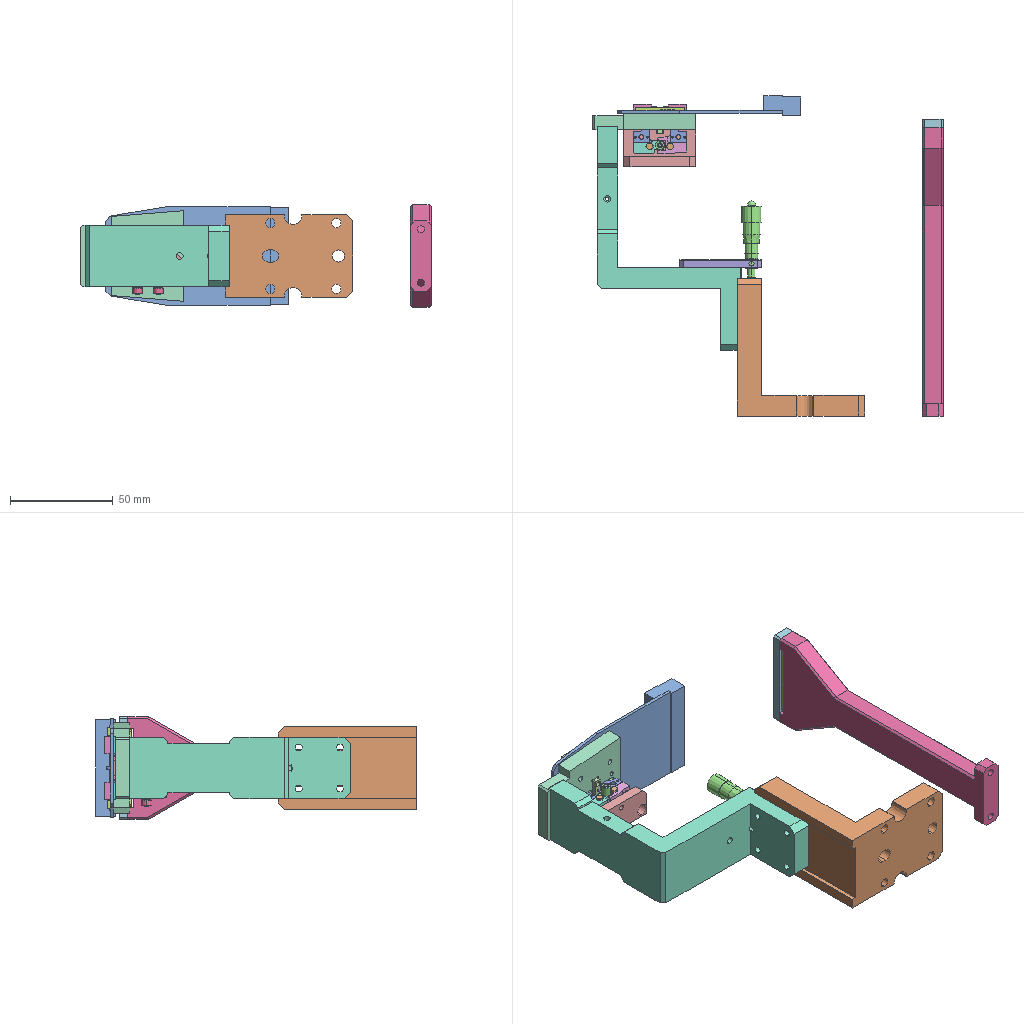Assembly | SolidWorks | 33 different items | 55 placed | box 170 x 156 x 50 mm
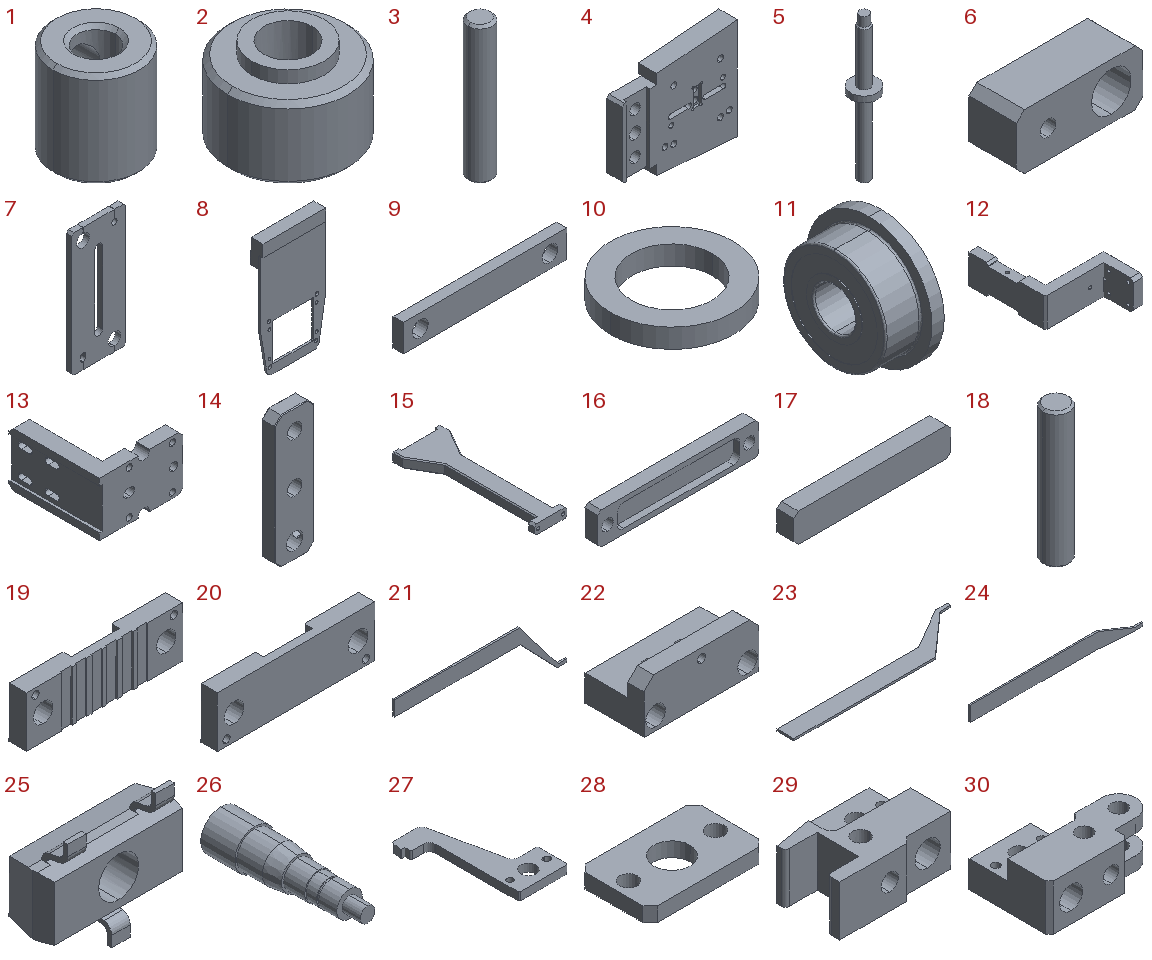Parts list (item | quantity | size | volume | features):
1 | x1 | 4.5 x 4.5 x 5 mm | 60.379 mm3 | features Chamfer 1, Extrusion 1, HoleWzd 1
2 | x2 | 5 x 5 x 3.5 mm | 47.704 mm3 | features Chamfer 1, Extrusion 1, HoleWzd 1, ICE 1
3 | x4 | 1 x 1 x 5.8 mm | 4.526 mm3 | features Chamfer 1, Extrusion 1
4 | x1 | 50 x 9.6 x 44 mm | 11717 mm3 | features HoleWzd 10, ICE 8, Chamfer 2, Cut 1, Extrusion 1
5 | x1 | 2.3 x 2.3 x 12.4 mm | 11.168 mm3 | features ICE 3, Chamfer 1, Extrusion 1
6 | x1 | 8 x 3 x 3.5 mm | 57.171 mm3 | features HoleWzd 2, Chamfer 1, Extrusion 1, ICE 1
7 | x1 | 12 x 1.2 x 27.5 mm | 338.908 mm3 | features ICE 3, HoleWzd 2, Chamfer 1, Extrusion 1
8 | x1 | 48 x 9.5 x 89 mm | 10809 mm3 | features ICE 5, HoleWzd 2, LPattern 2, Chamfer 1, Cut 1, Extrusion 1, Fillet 1
9 | x2 | 24 x 1.5 x 4 mm | 131.536 mm3 | features Extrusion 1, HoleWzd 1
10 | x2 | 3.2 x 3.2 x 0.5 mm | 2.289 mm3 | features Extrusion 1
11 | x4 | 2.3 x 6.1 x 6.1 mm | 42.794 mm3 | features BaseBody 1
12 | x1 | 70 x 108.5 x 30 mm | 47415 mm3 | features Chamfer 5, HoleWzd 4, ICE 4, Extrusion 1, MirrorPattern 1
13 | x1 | 62 x 67 x 40 mm | 44252 mm3 | features ICE 4, Chamfer 1, Cut 1, Extrusion 1, HoleWzd 1
14 | x1 | 12 x 4 x 40 mm | 1661 mm3 | features HoleWzd 3, Chamfer 2, Extrusion 1
15 | x1 | 50 x 140 x 10 mm | 32128 mm3 | features Chamfer 2, HoleWzd 2, ICE 2, Extrusion 1, MirrorPattern 1
16 | x1 | 50 x 4 x 10 mm | 1390 mm3 | features Chamfer 1, Extrusion 1, HoleWzd 1, ICE 1
17 | x1 | 37 x 4 x 6.8 mm | 998.4 mm3 | features Chamfer 1, Extrusion 1
18 | x6 | 1.2 x 1.2 x 6.2 mm | 6.976 mm3 | features Chamfer 1, Extrusion 1
19 | x2 | 25.7 x 2.85 x 8.3 mm | 448.741 mm3 | features ICE 3, Chamfer 1, Extrusion 1
20 | x2 | 25.7 x 2.65 x 8.3 mm | 426.68 mm3 | features Chamfer 1, Extrusion 1, ICE 1
21 | x2 | 19.5 x 0.2 x 6.07 mm | 5.761 mm3 | features Extrusion 1
22 | x1 | 35 x 18 x 15 mm | 5316 mm3 | features HoleWzd 4, Chamfer 1, Extrusion 1, ICE 1
23 | x2 | 19.5 x 4.08 x 0.2 mm | 5.788 mm3 | features Extrusion 1
24 | x2 | 19.5 x 0.2 x 2.02 mm | 5.825 mm3 | features Extrusion 1
25 | x1 | 2.908 x 1.057 x 2.408 mm | 2.992 mm3 | features ICE 6, Fillet 4, Extrusion 1, RefAxis 1
26 | x1 | 9.4 x 37 x 9.4 mm | 1530 mm3 | features ICE 7, Chamfer 1, Extrusion 1, Fillet 1
27 | x2 | 11.6 x 17.5 x 1.3 mm | 99.407 mm3 | features ICE 4, Fillet 3, Chamfer 1, Extrusion 1
28 | x2 | 8 x 5 x 1 mm | 32.329 mm3 | features Chamfer 1, Extrusion 1, ICE 1
29 | x1 | 14 x 10.5 x 6 mm | 468.744 mm3 | features HoleWzd 5, ICE 4, Fillet 2, Extrusion 1
30 | x1 | 15.25 x 10.5 x 6 mm | 471.852 mm3 | features HoleWzd 5, ICE 5, Fillet 2, Chamfer 1, Extrusion 1
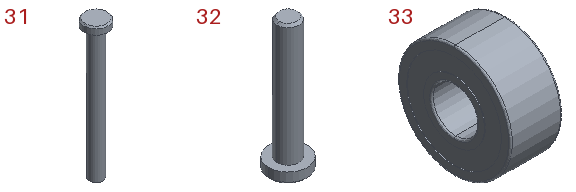31 | x2 | 3.5 x 3.5 x 20.5 mm | 69.56 mm3 | features ICE 3, Chamfer 1, Extrusion 1
32 | x1 | 3.5 x 3.5 x 12 mm | 43.298 mm3 | features ICE 2, Chamfer 1, Extrusion 1
33 | x1 | 2.3 x 5 x 5 mm | 37.258 mm3 | features BaseBody 1
Mates (type | each side: item.copy, entity, surface, feature):
Coincident | 28.1 face plane Boss-Extrude1 | 29.1 face plane Cut-Extrude1
Concentric | 28.1 face cylinder Cut-Extrude1 | 29.1 face cylinder Ø1.0 (1) Diameter Hole1
Concentric | 28.1 face cylinder Cut-Extrude1 | 29.1 face cylinder M2.5 Tapped Hole1
Coincident | 27.1 face plane Boss-Extrude1 | 28.1 face plane Boss-Extrude1
Concentric | 27.1 face cylinder Cut-Extrude1 | 28.1 face cylinder Cut-Extrude1 | 2 times
Coincident | 28.2 face plane Boss-Extrude1 | 30.1 face plane Cut-Extrude1
Concentric | 28.2 face cylinder Cut-Extrude1 | 30.1 face cylinder M2.5 Tapped Hole1
Concentric | 28.2 face cylinder Cut-Extrude1 | 30.1 face cylinder Ø1.0 (1) Diameter Hole1
Coincident | 27.2 face plane Boss-Extrude1 | 28.2 face plane Boss-Extrude1
Concentric | 27.2 face cylinder Cut-Extrude1 | 28.2 face cylinder Cut-Extrude1
Concentric | 27.2 face cylinder Cut-Extrude1 | 30.1 face cylinder Ø1.0 (1) Diameter Hole1
Concentric | 30.1 face cylinder Ø2.0 (2) Diameter Hole1 | 31.1 face cylinder Boss-Extrude1
Coincident | 30.1 face plane Boss-Extrude1 | 31.1 face plane Boss-Extrude2
Concentric | 29.1 face cylinder Ø2.0 (2) Diameter Hole1 | 31.2 face cylinder Boss-Extrude1
Coincident | 29.1 face plane Boss-Extrude1 | 31.2 face plane Boss-Extrude2
Width | 33.1 face plane Input1 | 33.1 face plane Input1 | 30.1 face plane Cut-Extrude5 | 30.1 face plane Cut-Extrude5
Concentric | 30.1 face cylinder Cut-Extrude4 | 33.1 face cylinder Input1
Concentric | 30.1 face cylinder Cut-Extrude4 | 32.1 face cylinder Boss-Extrude2
Coincident | 30.1 face plane Boss-Extrude1 | 32.1 face plane Boss-Extrude1
Concentric | 32.1 face cylinder Boss-Extrude2 | 1.1 face cylinder Boss-Extrude1
Coincident | 32.1 face plane Boss-Extrude2 | 1.1 face plane Boss-Extrude1
Concentric | 22.1 face cylinder Ø5.0 (5) Diameter Hole1 | 11.1 face cylinder Input1
Coincident | 22.1 face plane Boss-Extrude1 | 11.1 face plane Input1
Concentric | 22.1 face cylinder Ø5.0 (5) Diameter Hole1 | 11.2 face cylinder Input1
Coincident | 22.1 face plane Cut-Extrude1 | 11.2 face plane Input1
Concentric | 22.1 face cylinder Ø5.0 (5) Diameter Hole1 | 11.3 face cylinder Input1
Coincident | 22.1 face plane Boss-Extrude1 | 11.3 face plane Input1
Concentric | 22.1 face cylinder Ø5.0 (5) Diameter Hole1 | 11.4 face cylinder Input1
Coincident | 22.1 face plane Cut-Extrude1 | 11.4 face plane Input1
Concentric | 31.2 face cylinder Boss-Extrude1 | 11.2 face cylinder Input1
Coincident | 10.1 face plane Boss-Extrude1 | 11.2 face plane Input1
Concentric | 31.1 face cylinder Boss-Extrude1 | 11.4 face cylinder Input1
Coincident | 10.2 face plane Boss-Extrude1 | 11.4 face plane Input1
Coincident | 2.1 face plane Boss-Extrude2 | 11.3 face plane Input1
Concentric | 31.1 face cylinder Boss-Extrude1 | 2.1 face cylinder Boss-Extrude1
Coincident | 2.2 face plane Boss-Extrude2 | 11.1 face plane Input1
Concentric | 31.2 face cylinder Boss-Extrude1 | 2.2 face cylinder Boss-Extrude1
Tangent | 29.1 face plane Cut-Extrude3 | 33.1 face cylinder Input1 | 2 times
Coincident | 30.1 face plane Boss-Extrude1 | 3.1 face plane Boss-Extrude1
Coincident | 30.1 face plane Boss-Extrude1 | 3.2 face plane Boss-Extrude1
Coincident | 29.1 face plane Boss-Extrude1 | 3.3 face plane Boss-Extrude1
Coincident | 29.1 face plane Boss-Extrude1 | 3.4 face plane Boss-Extrude1
Concentric | 29.1 face cylinder Ø1.0 (1) Diameter Hole1 | 3.4 face cylinder Boss-Extrude1
Concentric | 29.1 face cylinder Ø1.0 (1) Diameter Hole1 | 3.3 face cylinder Boss-Extrude1
Concentric | 30.1 face cylinder Ø1.0 (1) Diameter Hole1 | 3.2 face cylinder Boss-Extrude1
Concentric | 30.1 face cylinder Ø1.0 (1) Diameter Hole1 | 3.1 face cylinder Boss-Extrude1
Coincident | 22.1 face plane Boss-Extrude1 | 4.1 face plane Boss-Extrude1
Width | 4.1 face plane Boss-Extrude1 | 4.1 face plane Boss-Extrude1 | 22.1 face plane Boss-Extrude1 | 22.1 face plane Boss-Extrude1
Width | 4.1 face plane Cut-Extrude7 | 4.1 face plane Cut-Extrude7 | 27.1 face plane Boss-Extrude1 | 27.1 face plane Boss-Extrude1
Width | 25.1 face plane Cut-Extrude1 | 25.1 face plane Cut-Extrude1 | 4.1 face plane Boss-Extrude2 | 4.1 face plane Boss-Extrude2
Width | 25.1 face plane Cut-Extrude3 | 25.1 face plane Cut-Extrude3 | 4.1 face plane Boss-Extrude2 | 4.1 face plane Boss-Extrude2
Coincident | 4.1 face plane Boss-Extrude2 | 25.1 face plane Boss-Extrude1
Concentric | 4.1 face cylinder Ø1.2 (1.2) Diameter Hole1 | 5.1 face cylinder Boss-Extrude2
Coincident | 4.1 face plane Cut-Extrude3 | 5.1 face plane Boss-Extrude1
Coincident | 4.1 face plane Cut-Extrude4 | 6.1 face plane Boss-Extrude1 | 2 times
Concentric | 4.1 face cylinder Cut-Extrude3 | 6.1 face cylinder Cut-Extrude1
Width | 4.1 face plane Boss-Extrude1 | 4.1 face plane Boss-Extrude1 | 7.1 face plane Boss-Extrude1 | 7.1 face plane Boss-Extrude1
Coincident | 4.1 face plane Cut-Extrude6 | 7.1 face plane Boss-Extrude1
Coincident | 29.1 face plane Boss-Extrude1 | 30.1 face plane Boss-Extrude1
DistanceDim | 4.1 face plane Boss-Extrude1 | 8.1 face plane Boss-Extrude1
Width | 4.1 face plane Cut-Extrude7 | 4.1 face plane Cut-Extrude7 | 8.1 face plane Boss-Extrude1 | 8.1 face plane Boss-Extrude1
Coincident | 4.1 face plane Boss-Extrude1 | 8.1 face plane Boss-Extrude1
Coincident | 8.1 face plane Boss-Extrude1 | 9.1 face plane Boss-Extrude1
Coincident | 8.1 face plane Boss-Extrude1 | 9.2 face plane Boss-Extrude1
Width | 4.1 face plane Cut-Extrude7 | 4.1 face plane Cut-Extrude7 | 12.1 face plane Boss-Extrude1 | 12.1 face plane Boss-Extrude1
Coincident | 12.1 face plane Boss-Extrude1 | 13.1 face plane Cut-Extrude2 | 2 times
DistanceDim | 13.1 face plane Boss-Extrude1 | 12.1 face plane Boss-Extrude1
Coincident | 14.1 face plane Boss-Extrude1 | 12.1 face plane Boss-Extrude1
Concentric | 14.1 face cylinder M6 Tapped Hole1 | 26.1 face cylinder Boss-Extrude2
Coincident | 14.1 face plane Boss-Extrude1 | 26.1 face plane Boss-Extrude2
Concentric | 12.1 face cylinder M4 Tapped Hole1 | 14.1 face cylinder Ø4.5 (4.5) Diameter Hole1 | 2 times
DistanceDim | 13.1 face plane Boss-Extrude1 | 15.1 face plane Boss-Extrude1
Width | 13.1 face plane Boss-Extrude1 | 13.1 face plane Boss-Extrude1 | 15.1 face plane Mirror1 | 15.1 face plane Cut-Extrude1
Coincident | 13.1 face plane Boss-Extrude1 | 15.1 face plane Boss-Extrude1
Coincident | 15.1 face plane Boss-Extrude1 | 16.1 face plane Boss-Extrude1
Concentric | 15.1 face cylinder M3 Tapped Hole1 | 16.1 face cylinder Ø3.5 (3.5) Diameter Hole1 | 2 times
Width | 16.1 face plane Cut-Extrude1 | 16.1 face plane Cut-Extrude1 | 17.1 face plane Boss-Extrude1 | 17.1 face plane Boss-Extrude1
DistanceDim | 16.1 face plane Cut-Extrude1 | 17.1 face plane Boss-Extrude1
Coincident | 16.1 face plane Cut-Extrude1 | 17.1 face plane Boss-Extrude1
Coincident | 4.1 edge | 18.1 face plane Boss-Extrude1
Concentric | 4.1 face cylinder Ø1.2 (1.2) Diameter Hole2 | 18.1 face cylinder Boss-Extrude1
Coincident | 18.1 face plane Boss-Extrude1 | 18.2 face plane Boss-Extrude1
Concentric | 4.1 face cylinder Ø1.2 (1.2) Diameter Hole2 | 18.2 face cylinder Boss-Extrude1
Coincident | 18.3 face plane Boss-Extrude1 | 18.4 face plane Boss-Extrude1
Coincident | 18.4 face plane Boss-Extrude1 | 18.5 face plane Boss-Extrude1
Coincident | 18.5 face plane Boss-Extrude1 | 18.6 face plane Boss-Extrude1
Coincident | 18.1 face plane Boss-Extrude1 | 18.3 face plane Boss-Extrude1
Concentric | 4.1 face cylinder Ø1.2 (1.2) Diameter Hole2 | 18.3 face cylinder Boss-Extrude1
Concentric | 4.1 face cylinder Ø1.2 (1.2) Diameter Hole2 | 18.4 face cylinder Boss-Extrude1
Concentric | 4.1 face cylinder Ø1.2 (1.2) Diameter Hole2 | 18.5 face cylinder Boss-Extrude1
Concentric | 4.1 face cylinder Ø1.2 (1.2) Diameter Hole2 | 18.6 face cylinder Boss-Extrude1
Coincident | 4.1 face plane Cut-Extrude8 | 12.1 face plane Boss-Extrude2
Coincident | 4.1 face plane Boss-Extrude3 | 12.1 face plane Boss-Extrude1
Coincident | 4.1 face plane Cut-Extrude8 | 12.1 face plane Boss-Extrude1
Coincident | 30.1 face plane Boss-Extrude1 | 10.2 face plane Boss-Extrude1
Concentric | 31.1 face cylinder Boss-Extrude1 | 10.2 face cylinder Boss-Extrude1
Coincident | 29.1 face plane Boss-Extrude1 | 10.1 face plane Boss-Extrude1
Concentric | 31.2 face cylinder Boss-Extrude1 | 10.1 face cylinder Boss-Extrude1
Coincident | 19.1 face plane Boss-Extrude1 | 20.1 face plane Boss-Extrude1 | 3 times
Coincident | 19.1 face plane Cut-Extrude2 | 21.1 face plane Boss-Extrude1 | 2 times
Coincident | 19.1 face plane Cut-Extrude2 | 23.1 face plane Boss-Extrude1 | 2 times
Coincident | 19.1 face plane Cut-Extrude2 | 24.1 face plane Boss-Extrude1 | 2 times
DistanceDim | 21.1 face plane Boss-Extrude1 | 20.1 face plane Boss-Extrude1
Coincident | 21.1 face plane Boss-Extrude1 | 23.1 face plane Boss-Extrude1
Coincident | 23.1 face plane Boss-Extrude1 | 24.1 face plane Boss-Extrude1
DistanceDim | 19.1 face plane Boss-Extrude1 | 9.2 face plane Boss-Extrude1
Width | 9.2 face plane Boss-Extrude1 | 9.2 face plane Boss-Extrude1 | 19.1 face plane Boss-Extrude1 | 19.1 face plane Boss-Extrude1
Width | 20.1 face plane Boss-Extrude1 | 20.1 face plane Boss-Extrude1 | 4.1 face plane Boss-Extrude1 | 4.1 face plane Boss-Extrude1
Coincident | 4.1 face plane Cut-Extrude6 | 20.1 face plane Boss-Extrude1 | 2 times
Coincident | 19.2 face plane Boss-Extrude1 | 20.2 face plane Boss-Extrude1 | 3 times
Coincident | 19.2 face plane Cut-Extrude2 | 21.2 face plane Boss-Extrude1 | 2 times
Coincident | 19.2 face plane Cut-Extrude2 | 23.2 face plane Boss-Extrude1 | 2 times
Coincident | 19.2 face plane Cut-Extrude2 | 24.2 face plane Boss-Extrude1 | 2 times
DistanceDim | 21.2 face plane Boss-Extrude1 | 20.2 face plane Boss-Extrude1
Coincident | 21.2 face plane Boss-Extrude1 | 23.2 face plane Boss-Extrude1
Coincident | 23.2 face plane Boss-Extrude1 | 24.2 face plane Boss-Extrude1
DistanceDim | 19.2 face plane Boss-Extrude1 | 9.1 face plane Boss-Extrude1
Width | 9.1 face plane Boss-Extrude1 | 9.1 face plane Boss-Extrude1 | 19.2 face plane Boss-Extrude1 | 19.2 face plane Boss-Extrude1
Coincident | 4.1 face plane Cut-Extrude6 | 20.2 face plane Boss-Extrude1 | 2 times
Width | 20.2 face plane Boss-Extrude1 | 20.2 face plane Boss-Extrude1 | 4.1 face plane Boss-Extrude1 | 4.1 face plane Boss-Extrude1